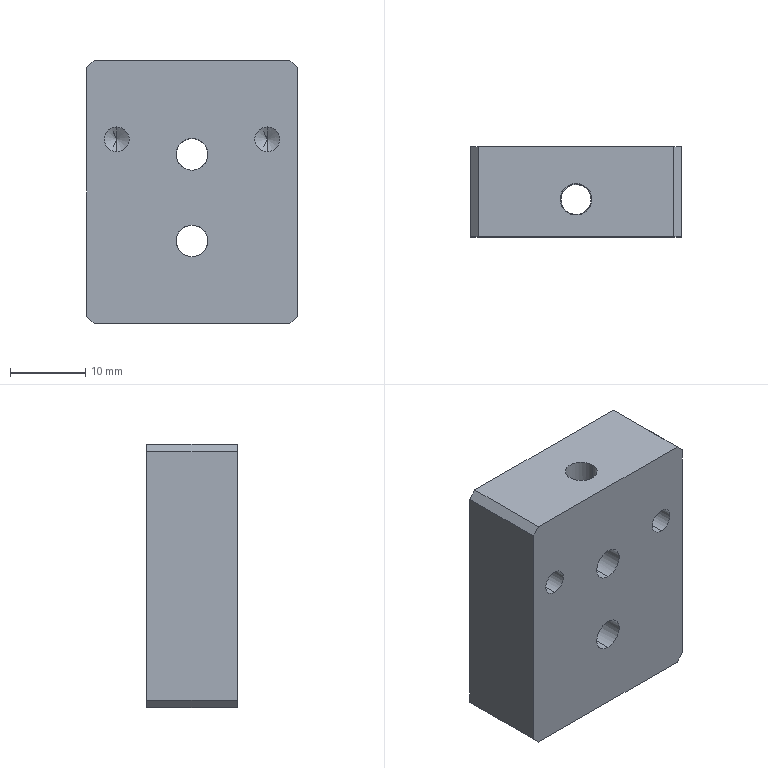Part | STEP file | 11-FG-E04411 | 1 solid | 36 faces | box 28 x 12 x 35 mm | volume 10850 mm3 | cylinder 19 | plane 10 | cone 7 | commonest cylinder face diameters 4.2 x13 3.3 x4 4 x2
STEP:
#1=CARTESIAN_POINT('',(-2.099,5.,5.1));
#2=VERTEX_POINT('',#1);
#3=CARTESIAN_POINT('',(-2.098,4.9,5.1));
#4=VERTEX_POINT('',#3);
#5=CARTESIAN_POINT('',(-2.099,5.,5.1));
#6=CARTESIAN_POINT('',(-2.098,4.967,5.1));
#7=CARTESIAN_POINT('',(-2.098,4.933,5.1));
#8=CARTESIAN_POINT('',(-2.098,4.9,5.1));
#9=B_SPLINE_CURVE_WITH_KNOTS('',3,(#5,#6,#7,#8),.UNSPECIFIED.,.F.,.F.,(4,4),(0.5,1.),.UNSPECIFIED.);
#10=EDGE_CURVE('',#2,#4,#9,.T.);
#11=ORIENTED_EDGE('',*,*,#10,.F.);
#12=CARTESIAN_POINT('',(-2.1,5.,17.5));
#13=VERTEX_POINT('',#12);
#14=CARTESIAN_POINT('',(-2.1,5.,17.5));
#15=DIRECTION('',(0.,0.,1.));
#16=VECTOR('',#15,1000.);
#17=LINE('',#14,#16);
#18=EDGE_CURVE('',#2,#13,#17,.T.);
#19=ORIENTED_EDGE('',*,*,#18,.T.);
#20=CARTESIAN_POINT('',(2.1,5.,17.5));
#21=VERTEX_POINT('',#20);
#22=CARTESIAN_POINT('',(0.,5.,17.5));
#23=DIRECTION('',(0.,0.,1.));
#24=DIRECTION('',(1.,0.,0.));
#25=AXIS2_PLACEMENT_3D('',#22,#23,#24);
#26=CIRCLE('',#25,2.1);
#27=EDGE_CURVE('',#13,#21,#26,.T.);
#28=ORIENTED_EDGE('',*,*,#27,.T.);
#29=CARTESIAN_POINT('',(2.099,5.,5.1));
#30=VERTEX_POINT('',#29);
#31=CARTESIAN_POINT('',(2.1,5.,17.5));
#32=DIRECTION('',(0.,0.,1.));
#33=VECTOR('',#32,1000.);
#34=LINE('',#31,#33);
#35=EDGE_CURVE('',#30,#21,#34,.T.);
#36=ORIENTED_EDGE('',*,*,#35,.F.);
#37=CARTESIAN_POINT('',(2.098,4.9,5.1));
#38=VERTEX_POINT('',#37);
#39=CARTESIAN_POINT('',(2.098,4.9,5.1));
#40=CARTESIAN_POINT('',(2.098,4.933,5.1));
#41=CARTESIAN_POINT('',(2.098,4.967,5.1));
#42=CARTESIAN_POINT('',(2.099,5.,5.1));
#43=B_SPLINE_CURVE_WITH_KNOTS('',3,(#39,#40,#41,#42),.UNSPECIFIED.,.F.,.F.,(4,4),(0.,0.5),.UNSPECIFIED.);
#44=EDGE_CURVE('',#38,#30,#43,.T.);
#45=ORIENTED_EDGE('',*,*,#44,.F.);
#46=CARTESIAN_POINT('',(0.,2.9,7.1));
#47=VERTEX_POINT('',#46);
#48=CARTESIAN_POINT('',(0.,2.9,7.1));
#49=CARTESIAN_POINT('',(1.184,2.9,7.1));
#50=CARTESIAN_POINT('',(2.041,3.717,6.283));
#51=CARTESIAN_POINT('',(2.098,4.9,5.1));
#52=(BOUNDED_CURVE()B_SPLINE_CURVE(3,(#48,#49,#50,#51),.UNSPECIFIED.,.F.,.F.)B_SPLINE_CURVE_WITH_KNOTS((4,4),(3.142,4.665),.UNSPECIFIED.)CURVE()GEOMETRIC_REPRESENTATION_ITEM()RATIONAL_B_SPLINE_CURVE((1.,0.8158,0.8158,1.))REPRESENTATION_ITEM(''));
#53=EDGE_CURVE('',#47,#38,#52,.T.);
#54=ORIENTED_EDGE('',*,*,#53,.F.);
#55=CARTESIAN_POINT('',(-2.098,4.9,5.1));
#56=CARTESIAN_POINT('',(-2.041,3.717,6.283));
#57=CARTESIAN_POINT('',(-1.184,2.9,7.1));
#58=CARTESIAN_POINT('',(0.,2.9,7.1));
#59=(BOUNDED_CURVE()B_SPLINE_CURVE(3,(#55,#56,#57,#58),.UNSPECIFIED.,.F.,.F.)B_SPLINE_CURVE_WITH_KNOTS((4,4),(1.618,3.142),.UNSPECIFIED.)CURVE()GEOMETRIC_REPRESENTATION_ITEM()RATIONAL_B_SPLINE_CURVE((1.,0.8158,0.8158,1.))REPRESENTATION_ITEM(''));
#60=EDGE_CURVE('',#4,#47,#59,.T.);
#61=ORIENTED_EDGE('',*,*,#60,.F.);
#62=EDGE_LOOP('',(#11,#19,#28,#36,#45,#54,#61));
#63=FACE_OUTER_BOUND('',#62,.T.);
#64=CARTESIAN_POINT('',(0.,5.,17.5));
#65=DIRECTION('',(0.,0.,1.));
#66=DIRECTION('',(1.,0.,0.));
#67=AXIS2_PLACEMENT_3D('',#64,#65,#66);
#68=CYLINDRICAL_SURFACE('',#67,2.1);
#69=ADVANCED_FACE('',(#63),#68,.F.);
#70=CARTESIAN_POINT('',(2.1,5.,-6.5));
#71=VERTEX_POINT('',#70);
#72=CARTESIAN_POINT('',(0.,2.9,-8.6));
#73=VERTEX_POINT('',#72);
#74=CARTESIAN_POINT('',(2.1,5.,-6.5));
#75=CARTESIAN_POINT('',(2.1,3.77,-7.73));
#76=CARTESIAN_POINT('',(1.23,2.9,-8.6));
#77=CARTESIAN_POINT('',(0.,2.9,-8.6));
#78=(BOUNDED_CURVE()B_SPLINE_CURVE(3,(#74,#75,#76,#77),.UNSPECIFIED.,.F.,.F.)B_SPLINE_CURVE_WITH_KNOTS((4,4),(1.571,3.142),.UNSPECIFIED.)CURVE()GEOMETRIC_REPRESENTATION_ITEM()RATIONAL_B_SPLINE_CURVE((1.,0.8047,0.8047,1.))REPRESENTATION_ITEM(''));
#79=EDGE_CURVE('',#71,#73,#78,.T.);
#80=ORIENTED_EDGE('',*,*,#79,.F.);
#81=CARTESIAN_POINT('',(2.1,5.,-17.5));
#82=VERTEX_POINT('',#81);
#83=CARTESIAN_POINT('',(2.1,5.,-17.5));
#84=DIRECTION('',(0.,0.,-1.));
#85=VECTOR('',#84,1000.);
#86=LINE('',#83,#85);
#87=EDGE_CURVE('',#71,#82,#86,.T.);
#88=ORIENTED_EDGE('',*,*,#87,.T.);
#89=CARTESIAN_POINT('',(-2.1,5.,-17.5));
#90=VERTEX_POINT('',#89);
#91=CARTESIAN_POINT('',(0.,5.,-17.5));
#92=DIRECTION('',(0.,0.,-1.));
#93=DIRECTION('',(-1.,0.,0.));
#94=AXIS2_PLACEMENT_3D('',#91,#92,#93);
#95=CIRCLE('',#94,2.1);
#96=EDGE_CURVE('',#82,#90,#95,.T.);
#97=ORIENTED_EDGE('',*,*,#96,.T.);
#98=CARTESIAN_POINT('',(-2.1,5.,-6.5));
#99=VERTEX_POINT('',#98);
#100=CARTESIAN_POINT('',(-2.1,5.,-17.5));
#101=DIRECTION('',(0.,0.,-1.));
#102=VECTOR('',#101,1000.);
#103=LINE('',#100,#102);
#104=EDGE_CURVE('',#99,#90,#103,.T.);
#105=ORIENTED_EDGE('',*,*,#104,.F.);
#106=CARTESIAN_POINT('',(0.,2.9,-8.6));
#107=CARTESIAN_POINT('',(-1.23,2.9,-8.6));
#108=CARTESIAN_POINT('',(-2.1,3.77,-7.73));
#109=CARTESIAN_POINT('',(-2.1,5.,-6.5));
#110=(BOUNDED_CURVE()B_SPLINE_CURVE(3,(#106,#107,#108,#109),.UNSPECIFIED.,.F.,.T.)B_SPLINE_CURVE_WITH_KNOTS((4,4),(3.142,4.712),.UNSPECIFIED.)CURVE()GEOMETRIC_REPRESENTATION_ITEM()RATIONAL_B_SPLINE_CURVE((1.,0.8047,0.8047,1.))REPRESENTATION_ITEM(''));
#111=EDGE_CURVE('',#73,#99,#110,.T.);
#112=ORIENTED_EDGE('',*,*,#111,.F.);
#113=EDGE_LOOP('',(#80,#88,#97,#105,#112));
#114=FACE_OUTER_BOUND('',#113,.T.);
#115=CARTESIAN_POINT('',(0.,5.,-17.5));
#116=DIRECTION('',(0.,0.,-1.));
#117=DIRECTION('',(-1.,0.,0.));
#118=AXIS2_PLACEMENT_3D('',#115,#116,#117);
#119=CYLINDRICAL_SURFACE('',#118,2.1);
#120=ADVANCED_FACE('',(#114),#119,.F.);
#121=CARTESIAN_POINT('',(-2.1,5.,-5.1));
#122=VERTEX_POINT('',#121);
#123=CARTESIAN_POINT('',(-1.565,6.4,-5.1));
#124=VERTEX_POINT('',#123);
#125=CARTESIAN_POINT('',(0.,5.,-5.1));
#126=DIRECTION('',(0.,0.,-1.));
#127=DIRECTION('',(-1.,0.,0.));
#128=AXIS2_PLACEMENT_3D('',#125,#126,#127);
#129=CIRCLE('',#128,2.1);
#130=EDGE_CURVE('',#122,#124,#129,.T.);
#131=ORIENTED_EDGE('',*,*,#130,.F.);
#132=CARTESIAN_POINT('',(-2.1,5.,-17.5));
#133=DIRECTION('',(0.,0.,-1.));
#134=VECTOR('',#133,1000.);
#135=LINE('',#132,#134);
#136=EDGE_CURVE('',#122,#99,#135,.T.);
#137=ORIENTED_EDGE('',*,*,#136,.T.);
#138=CARTESIAN_POINT('',(-1.565,6.4,-5.1));
#139=CARTESIAN_POINT('',(-1.914,6.011,-5.489));
#140=CARTESIAN_POINT('',(-2.1,5.522,-5.978));
#141=CARTESIAN_POINT('',(-2.1,5.,-6.5));
#142=(BOUNDED_CURVE()B_SPLINE_CURVE(3,(#138,#139,#140,#141),.UNSPECIFIED.,.F.,.F.)B_SPLINE_CURVE_WITH_KNOTS((4,4),(0.8411,1.571),.UNSPECIFIED.)CURVE()GEOMETRIC_REPRESENTATION_ITEM()RATIONAL_B_SPLINE_CURVE((1.,0.9561,0.9561,1.))REPRESENTATION_ITEM(''));
#143=EDGE_CURVE('',#124,#99,#142,.T.);
#144=ORIENTED_EDGE('',*,*,#143,.F.);
#145=EDGE_LOOP('',(#131,#137,#144));
#146=FACE_OUTER_BOUND('',#145,.T.);
#147=CARTESIAN_POINT('',(0.,5.,-17.5));
#148=DIRECTION('',(0.,0.,-1.));
#149=DIRECTION('',(-1.,0.,0.));
#150=AXIS2_PLACEMENT_3D('',#147,#148,#149);
#151=CYLINDRICAL_SURFACE('',#150,2.1);
#152=ADVANCED_FACE('',(#146),#151,.F.);
#153=CARTESIAN_POINT('',(-2.,5.,-5.04));
#154=VERTEX_POINT('',#153);
#155=CARTESIAN_POINT('',(-1.509,6.312,-5.04));
#156=VERTEX_POINT('',#155);
#157=CARTESIAN_POINT('',(0.,5.,-5.04));
#158=DIRECTION('',(0.,0.,-1.));
#159=DIRECTION('',(-1.,0.,0.));
#160=AXIS2_PLACEMENT_3D('',#157,#158,#159);
#161=CIRCLE('',#160,2.);
#162=EDGE_CURVE('',#154,#156,#161,.T.);
#163=ORIENTED_EDGE('',*,*,#162,.F.);
#164=CARTESIAN_POINT('',(-2.1,5.,-5.1));
#165=DIRECTION('',(-0.8572,0.,-0.515));
#166=VECTOR('',#165,1000.);
#167=LINE('',#164,#166);
#168=EDGE_CURVE('',#154,#122,#167,.T.);
#169=ORIENTED_EDGE('',*,*,#168,.T.);
#170=ORIENTED_EDGE('',*,*,#130,.T.);
#171=CARTESIAN_POINT('',(-1.509,6.312,-5.04));
#172=CARTESIAN_POINT('',(-1.529,6.341,-5.06));
#173=CARTESIAN_POINT('',(-1.547,6.37,-5.08));
#174=CARTESIAN_POINT('',(-1.565,6.4,-5.1));
#175=B_SPLINE_CURVE_WITH_KNOTS('',3,(#171,#172,#173,#174),.UNSPECIFIED.,.F.,.F.,(4,4),(0.003861,0.00398),.UNSPECIFIED.);
#176=EDGE_CURVE('',#156,#124,#175,.T.);
#177=ORIENTED_EDGE('',*,*,#176,.F.);
#178=EDGE_LOOP('',(#163,#169,#170,#177));
#179=FACE_OUTER_BOUND('',#178,.T.);
#180=CARTESIAN_POINT('',(0.,5.,-5.1));
#181=DIRECTION('',(0.,0.,-1.));
#182=DIRECTION('',(-1.,0.,0.));
#183=AXIS2_PLACEMENT_3D('',#180,#181,#182);
#184=CONICAL_SURFACE('',#183,2.1,1.03);
#185=ADVANCED_FACE('',(#179),#184,.F.);
#186=CARTESIAN_POINT('',(2.,5.,4.36));
#187=VERTEX_POINT('',#186);
#188=CARTESIAN_POINT('',(0.,3.,2.9));
#189=VERTEX_POINT('',#188);
#190=CARTESIAN_POINT('',(2.,5.,4.36));
#191=CARTESIAN_POINT('',(2.,4.926,4.36));
#192=CARTESIAN_POINT('',(1.996,4.852,4.346));
#193=CARTESIAN_POINT('',(1.98,4.712,4.301));
#194=CARTESIAN_POINT('',(1.969,4.645,4.27));
#195=CARTESIAN_POINT('',(1.929,4.455,4.166));
#196=CARTESIAN_POINT('',(1.892,4.34,4.083));
#197=CARTESIAN_POINT('',(1.799,4.118,3.913));
#198=CARTESIAN_POINT('',(1.744,4.013,3.825));
#199=CARTESIAN_POINT('',(1.615,3.815,3.654));
#200=CARTESIAN_POINT('',(1.542,3.721,3.57));
#201=CARTESIAN_POINT('',(1.375,3.543,3.409));
#202=CARTESIAN_POINT('',(1.281,3.458,3.331));
#203=CARTESIAN_POINT('',(1.073,3.307,3.19));
#204=CARTESIAN_POINT('',(0.959,3.24,3.127));
#205=CARTESIAN_POINT('',(0.7085,3.125,3.018));
#206=CARTESIAN_POINT('',(0.5753,3.079,2.975));
#207=CARTESIAN_POINT('',(0.294,3.016,2.916));
#208=CARTESIAN_POINT('',(0.1462,3.,2.9));
#209=CARTESIAN_POINT('',(0.,3.,2.9));
#210=B_SPLINE_CURVE_WITH_KNOTS('',3,(#190,#191,#192,#193,#194,#195,#196,#197,#198,#199,#200,#201,#202,#203,#204,#205,#206,#207,#208,#209),.UNSPECIFIED.,.F.,.F.,(4,2,2,2,2,2,2,2,2,4),(0.007048,0.00727,0.007491,0.007933,0.008376,0.008818,0.009261,0.009703,0.01015,0.01059),.UNSPECIFIED.);
#211=EDGE_CURVE('',#187,#189,#210,.T.);
#212=ORIENTED_EDGE('',*,*,#211,.F.);
#213=CARTESIAN_POINT('',(2.,5.,-5.04));
#214=VERTEX_POINT('',#213);
#215=CARTESIAN_POINT('',(2.,5.,21.5));
#216=DIRECTION('',(0.,0.,-1.));
#217=VECTOR('',#216,1000.);
#218=LINE('',#215,#217);
#219=EDGE_CURVE('',#187,#214,#218,.T.);
#220=ORIENTED_EDGE('',*,*,#219,.T.);
#221=CARTESIAN_POINT('',(1.509,3.688,-5.04));
#222=VERTEX_POINT('',#221);
#223=CARTESIAN_POINT('',(0.,5.,-5.04));
#224=DIRECTION('',(0.,0.,-1.));
#225=DIRECTION('',(-1.,0.,0.));
#226=AXIS2_PLACEMENT_3D('',#223,#224,#225);
#227=CIRCLE('',#226,2.);
#228=EDGE_CURVE('',#214,#222,#227,.T.);
#229=ORIENTED_EDGE('',*,*,#228,.T.);
#230=CARTESIAN_POINT('',(0.,3.,-4.4));
#231=VERTEX_POINT('',#230);
#232=CARTESIAN_POINT('',(0.,3.,-4.4));
#233=CARTESIAN_POINT('',(0.1564,3.,-4.4));
#234=CARTESIAN_POINT('',(0.3081,3.018,-4.417));
#235=CARTESIAN_POINT('',(0.603,3.087,-4.483));
#236=CARTESIAN_POINT('',(0.7432,3.138,-4.531));
#237=CARTESIAN_POINT('',(1.001,3.262,-4.648));
#238=CARTESIAN_POINT('',(1.119,3.337,-4.718));
#239=CARTESIAN_POINT('',(1.331,3.501,-4.87));
#240=CARTESIAN_POINT('',(1.425,3.591,-4.953));
#241=CARTESIAN_POINT('',(1.509,3.688,-5.04));
#242=B_SPLINE_CURVE_WITH_KNOTS('',3,(#232,#233,#234,#235,#236,#237,#238,#239,#240,#241),.UNSPECIFIED.,.F.,.F.,(4,2,2,2,4),(0.,0.0004611,0.0009223,0.001383,0.001845),.UNSPECIFIED.);
#243=EDGE_CURVE('',#231,#222,#242,.T.);
#244=ORIENTED_EDGE('',*,*,#243,.F.);
#245=CARTESIAN_POINT('',(-1.509,3.688,-5.04));
#246=VERTEX_POINT('',#245);
#247=CARTESIAN_POINT('',(-1.509,3.688,-5.04));
#248=CARTESIAN_POINT('',(-1.425,3.591,-4.953));
#249=CARTESIAN_POINT('',(-1.331,3.501,-4.87));
#250=CARTESIAN_POINT('',(-1.119,3.337,-4.718));
#251=CARTESIAN_POINT('',(-1.,3.262,-4.648));
#252=CARTESIAN_POINT('',(-0.7433,3.138,-4.531));
#253=CARTESIAN_POINT('',(-0.6036,3.087,-4.483));
#254=CARTESIAN_POINT('',(-0.3082,3.018,-4.417));
#255=CARTESIAN_POINT('',(-0.1571,3.,-4.4));
#256=CARTESIAN_POINT('',(0.,3.,-4.4));
#257=B_SPLINE_CURVE_WITH_KNOTS('',3,(#247,#248,#249,#250,#251,#252,#253,#254,#255,#256),.UNSPECIFIED.,.F.,.F.,(4,2,2,2,4),(0.01221,0.01268,0.01314,0.0136,0.01407),.UNSPECIFIED.);
#258=EDGE_CURVE('',#246,#231,#257,.T.);
#259=ORIENTED_EDGE('',*,*,#258,.F.);
#260=CARTESIAN_POINT('',(0.,5.,-5.04));
#261=DIRECTION('',(0.,0.,-1.));
#262=DIRECTION('',(-1.,0.,0.));
#263=AXIS2_PLACEMENT_3D('',#260,#261,#262);
#264=CIRCLE('',#263,2.);
#265=EDGE_CURVE('',#246,#154,#264,.T.);
#266=ORIENTED_EDGE('',*,*,#265,.T.);
#267=CARTESIAN_POINT('',(-2.,5.,4.36));
#268=VERTEX_POINT('',#267);
#269=CARTESIAN_POINT('',(-2.,5.,21.5));
#270=DIRECTION('',(0.,0.,-1.));
#271=VECTOR('',#270,1000.);
#272=LINE('',#269,#271);
#273=EDGE_CURVE('',#268,#154,#272,.T.);
#274=ORIENTED_EDGE('',*,*,#273,.F.);
#275=CARTESIAN_POINT('',(0.,3.,2.9));
#276=CARTESIAN_POINT('',(-0.146,3.,2.9));
#277=CARTESIAN_POINT('',(-0.2945,3.017,2.916));
#278=CARTESIAN_POINT('',(-0.5747,3.079,2.975));
#279=CARTESIAN_POINT('',(-0.7099,3.125,3.019));
#280=CARTESIAN_POINT('',(-0.9584,3.239,3.127));
#281=CARTESIAN_POINT('',(-1.073,3.308,3.191));
#282=CARTESIAN_POINT('',(-1.282,3.46,3.332));
#283=CARTESIAN_POINT('',(-1.375,3.542,3.408));
#284=CARTESIAN_POINT('',(-1.542,3.72,3.569));
#285=CARTESIAN_POINT('',(-1.616,3.816,3.655));
#286=CARTESIAN_POINT('',(-1.745,4.016,3.827));
#287=CARTESIAN_POINT('',(-1.8,4.12,3.914));
#288=CARTESIAN_POINT('',(-1.892,4.34,4.083));
#289=CARTESIAN_POINT('',(-1.929,4.457,4.167));
#290=CARTESIAN_POINT('',(-1.983,4.711,4.306));
#291=CARTESIAN_POINT('',(-2.,4.85,4.36));
#292=CARTESIAN_POINT('',(-2.,5.,4.36));
#293=B_SPLINE_CURVE_WITH_KNOTS('',3,(#275,#276,#277,#278,#279,#280,#281,#282,#283,#284,#285,#286,#287,#288,#289,#290,#291,#292),.UNSPECIFIED.,.F.,.F.,(4,2,2,2,2,2,2,2,4),(0.01059,0.01103,0.01147,0.01191,0.01236,0.0128,0.01324,0.01368,0.01412),.UNSPECIFIED.);
#294=EDGE_CURVE('',#189,#268,#293,.T.);
#295=ORIENTED_EDGE('',*,*,#294,.F.);
#296=EDGE_LOOP('',(#212,#220,#229,#244,#259,#266,#274,#295));
#297=FACE_OUTER_BOUND('',#296,.T.);
#298=CARTESIAN_POINT('',(0.,5.,21.5));
#299=DIRECTION('',(0.,0.,-1.));
#300=DIRECTION('',(-1.,0.,0.));
#301=AXIS2_PLACEMENT_3D('',#298,#299,#300);
#302=CYLINDRICAL_SURFACE('',#301,2.);
#303=ADVANCED_FACE('',(#297),#302,.F.);
#304=CARTESIAN_POINT('',(-10.,10.1,8.65));
#305=VERTEX_POINT('',#304);
#306=CARTESIAN_POINT('',(-10.,10.1,5.35));
#307=VERTEX_POINT('',#306);
#308=CARTESIAN_POINT('',(-10.,10.1,7.));
#309=DIRECTION('',(0.,-1.,0.));
#310=DIRECTION('',(0.,0.,-1.));
#311=AXIS2_PLACEMENT_3D('',#308,#309,#310);
#312=CIRCLE('',#311,1.65);
#313=EDGE_CURVE('',#305,#307,#312,.T.);
#314=ORIENTED_EDGE('',*,*,#313,.F.);
#315=CARTESIAN_POINT('',(-10.,0.,8.65));
#316=VERTEX_POINT('',#315);
#317=CARTESIAN_POINT('',(-10.,0.,8.65));
#318=DIRECTION('',(0.,-1.,0.));
#319=VECTOR('',#318,1000.);
#320=LINE('',#317,#319);
#321=EDGE_CURVE('',#305,#316,#320,.T.);
#322=ORIENTED_EDGE('',*,*,#321,.T.);
#323=CARTESIAN_POINT('',(-10.,0.,5.35));
#324=VERTEX_POINT('',#323);
#325=CARTESIAN_POINT('',(-10.,0.,7.));
#326=DIRECTION('',(0.,-1.,0.));
#327=DIRECTION('',(0.,0.,-1.));
#328=AXIS2_PLACEMENT_3D('',#325,#326,#327);
#329=CIRCLE('',#328,1.65);
#330=EDGE_CURVE('',#316,#324,#329,.T.);
#331=ORIENTED_EDGE('',*,*,#330,.T.);
#332=CARTESIAN_POINT('',(-10.,0.,5.35));
#333=DIRECTION('',(0.,-1.,0.));
#334=VECTOR('',#333,1000.);
#335=LINE('',#332,#334);
#336=EDGE_CURVE('',#307,#324,#335,.T.);
#337=ORIENTED_EDGE('',*,*,#336,.F.);
#338=EDGE_LOOP('',(#314,#322,#331,#337));
#339=FACE_OUTER_BOUND('',#338,.T.);
#340=CARTESIAN_POINT('',(-10.,0.,7.));
#341=DIRECTION('',(0.,-1.,0.));
#342=DIRECTION('',(0.,0.,-1.));
#343=AXIS2_PLACEMENT_3D('',#340,#341,#342);
#344=CYLINDRICAL_SURFACE('',#343,1.65);
#345=ADVANCED_FACE('',(#339),#344,.F.);
#346=CARTESIAN_POINT('',(-10.,11.091,7.));
#347=VERTEX_POINT('',#346);
#348=CARTESIAN_POINT('',(-10.,10.1,5.35));
#349=DIRECTION('',(0.,-0.515,-0.8572));
#350=VECTOR('',#349,1000.);
#351=LINE('',#348,#350);
#352=EDGE_CURVE('',#347,#307,#351,.T.);
#353=ORIENTED_EDGE('',*,*,#352,.F.);
#354=CARTESIAN_POINT('',(-10.,10.1,8.65));
#355=DIRECTION('',(0.,-0.515,0.8572));
#356=VECTOR('',#355,1000.);
#357=LINE('',#354,#356);
#358=EDGE_CURVE('',#347,#305,#357,.T.);
#359=ORIENTED_EDGE('',*,*,#358,.T.);
#360=ORIENTED_EDGE('',*,*,#313,.T.);
#361=EDGE_LOOP('',(#353,#359,#360));
#362=FACE_OUTER_BOUND('',#361,.T.);
#363=CARTESIAN_POINT('',(-10.,10.1,7.));
#364=DIRECTION('',(0.,-1.,0.));
#365=DIRECTION('',(0.,0.,-1.));
#366=AXIS2_PLACEMENT_3D('',#363,#364,#365);
#367=CONICAL_SURFACE('',#366,1.65,1.03);
#368=ADVANCED_FACE('',(#362),#367,.F.);
#369=CARTESIAN_POINT('',(10.,10.1,8.65));
#370=VERTEX_POINT('',#369);
#371=CARTESIAN_POINT('',(10.,10.1,5.35));
#372=VERTEX_POINT('',#371);
#373=CARTESIAN_POINT('',(10.,10.1,7.));
#374=DIRECTION('',(0.,-1.,0.));
#375=DIRECTION('',(0.,0.,-1.));
#376=AXIS2_PLACEMENT_3D('',#373,#374,#375);
#377=CIRCLE('',#376,1.65);
#378=EDGE_CURVE('',#370,#372,#377,.T.);
#379=ORIENTED_EDGE('',*,*,#378,.F.);
#380=CARTESIAN_POINT('',(10.,0.,8.65));
#381=VERTEX_POINT('',#380);
#382=CARTESIAN_POINT('',(10.,0.,8.65));
#383=DIRECTION('',(0.,-1.,0.));
#384=VECTOR('',#383,1000.);
#385=LINE('',#382,#384);
#386=EDGE_CURVE('',#370,#381,#385,.T.);
#387=ORIENTED_EDGE('',*,*,#386,.T.);
#388=CARTESIAN_POINT('',(10.,0.,5.35));
#389=VERTEX_POINT('',#388);
#390=CARTESIAN_POINT('',(10.,0.,7.));
#391=DIRECTION('',(0.,-1.,0.));
#392=DIRECTION('',(0.,0.,-1.));
#393=AXIS2_PLACEMENT_3D('',#390,#391,#392);
#394=CIRCLE('',#393,1.65);
#395=EDGE_CURVE('',#381,#389,#394,.T.);
#396=ORIENTED_EDGE('',*,*,#395,.T.);
#397=CARTESIAN_POINT('',(10.,0.,5.35));
#398=DIRECTION('',(0.,-1.,0.));
#399=VECTOR('',#398,1000.);
#400=LINE('',#397,#399);
#401=EDGE_CURVE('',#372,#389,#400,.T.);
#402=ORIENTED_EDGE('',*,*,#401,.F.);
#403=EDGE_LOOP('',(#379,#387,#396,#402));
#404=FACE_OUTER_BOUND('',#403,.T.);
#405=CARTESIAN_POINT('',(10.,0.,7.));
#406=DIRECTION('',(0.,-1.,0.));
#407=DIRECTION('',(0.,0.,-1.));
#408=AXIS2_PLACEMENT_3D('',#405,#406,#407);
#409=CYLINDRICAL_SURFACE('',#408,1.65);
#410=ADVANCED_FACE('',(#404),#409,.F.);
#411=CARTESIAN_POINT('',(10.,11.091,7.));
#412=VERTEX_POINT('',#411);
#413=CARTESIAN_POINT('',(10.,10.1,5.35));
#414=DIRECTION('',(0.,-0.515,-0.8572));
#415=VECTOR('',#414,1000.);
#416=LINE('',#413,#415);
#417=EDGE_CURVE('',#412,#372,#416,.T.);
#418=ORIENTED_EDGE('',*,*,#417,.F.);
#419=CARTESIAN_POINT('',(10.,10.1,8.65));
#420=DIRECTION('',(0.,-0.515,0.8572));
#421=VECTOR('',#420,1000.);
#422=LINE('',#419,#421);
#423=EDGE_CURVE('',#412,#370,#422,.T.);
#424=ORIENTED_EDGE('',*,*,#423,.T.);
#425=ORIENTED_EDGE('',*,*,#378,.T.);
#426=EDGE_LOOP('',(#418,#424,#425));
#427=FACE_OUTER_BOUND('',#426,.T.);
#428=CARTESIAN_POINT('',(10.,10.1,7.));
#429=DIRECTION('',(0.,-1.,0.));
#430=DIRECTION('',(0.,0.,-1.));
#431=AXIS2_PLACEMENT_3D('',#428,#429,#430);
#432=CONICAL_SURFACE('',#431,1.65,1.03);
#433=ADVANCED_FACE('',(#427),#432,.F.);
#434=CARTESIAN_POINT('',(0.,7.1,-8.6));
#435=VERTEX_POINT('',#434);
#436=CARTESIAN_POINT('',(-2.1,5.,-6.5));
#437=CARTESIAN_POINT('',(-2.1,6.23,-7.73));
#438=CARTESIAN_POINT('',(-1.23,7.1,-8.6));
#439=CARTESIAN_POINT('',(0.,7.1,-8.6));
#440=(BOUNDED_CURVE()B_SPLINE_CURVE(3,(#436,#437,#438,#439),.UNSPECIFIED.,.F.,.F.)B_SPLINE_CURVE_WITH_KNOTS((4,4),(4.712,6.283),.UNSPECIFIED.)CURVE()GEOMETRIC_REPRESENTATION_ITEM()RATIONAL_B_SPLINE_CURVE((1.,0.8047,0.8047,1.))REPRESENTATION_ITEM(''));
#441=EDGE_CURVE('',#99,#435,#440,.T.);
#442=ORIENTED_EDGE('',*,*,#441,.T.);
#443=CARTESIAN_POINT('',(0.,12.,-8.6));
#444=VERTEX_POINT('',#443);
#445=CARTESIAN_POINT('',(0.,12.,-8.6));
#446=DIRECTION('',(0.,1.,0.));
#447=VECTOR('',#446,1000.);
#448=LINE('',#445,#447);
#449=EDGE_CURVE('',#435,#444,#448,.T.);
#450=ORIENTED_EDGE('',*,*,#449,.T.);
#451=CARTESIAN_POINT('',(0.,12.,-4.4));
#452=VERTEX_POINT('',#451);
#453=CARTESIAN_POINT('',(0.,12.,-6.5));
#454=DIRECTION('',(0.,1.,0.));
#455=DIRECTION('',(0.,0.,1.));
#456=AXIS2_PLACEMENT_3D('',#453,#454,#455);
#457=CIRCLE('',#456,2.1);
#458=EDGE_CURVE('',#444,#452,#457,.T.);
#459=ORIENTED_EDGE('',*,*,#458,.T.);
#460=CARTESIAN_POINT('',(0.,7.,-4.4));
#461=VERTEX_POINT('',#460);
#462=CARTESIAN_POINT('',(0.,12.,-4.4));
#463=DIRECTION('',(0.,1.,0.));
#464=VECTOR('',#463,1000.);
#465=LINE('',#462,#464);
#466=EDGE_CURVE('',#461,#452,#465,.T.);
#467=ORIENTED_EDGE('',*,*,#466,.F.);
#468=CARTESIAN_POINT('',(0.,7.,-4.4));
#469=CARTESIAN_POINT('',(-0.1553,7.,-4.4));
#470=CARTESIAN_POINT('',(-0.3073,6.982,-4.417));
#471=CARTESIAN_POINT('',(-0.6044,6.913,-4.483));
#472=CARTESIAN_POINT('',(-0.7426,6.863,-4.531));
#473=CARTESIAN_POINT('',(-1.002,6.737,-4.649));
#474=CARTESIAN_POINT('',(-1.119,6.663,-4.718));
#475=CARTESIAN_POINT('',(-1.33,6.5,-4.87));
#476=CARTESIAN_POINT('',(-1.426,6.408,-4.953));
#477=CARTESIAN_POINT('',(-1.509,6.312,-5.04));
#478=B_SPLINE_CURVE_WITH_KNOTS('',3,(#468,#469,#470,#471,#472,#473,#474,#475,#476,#477),.UNSPECIFIED.,.F.,.F.,(4,2,2,2,4),(0.007029,0.007491,0.007954,0.008416,0.008878),.UNSPECIFIED.);
#479=EDGE_CURVE('',#461,#156,#478,.T.);
#480=ORIENTED_EDGE('',*,*,#479,.T.);
#481=ORIENTED_EDGE('',*,*,#176,.T.);
#482=ORIENTED_EDGE('',*,*,#143,.T.);
#483=EDGE_LOOP('',(#442,#450,#459,#467,#480,#481,#482));
#484=FACE_OUTER_BOUND('',#483,.T.);
#485=CARTESIAN_POINT('',(0.,12.,-6.5));
#486=DIRECTION('',(0.,1.,0.));
#487=DIRECTION('',(0.,0.,1.));
#488=AXIS2_PLACEMENT_3D('',#485,#486,#487);
#489=CYLINDRICAL_SURFACE('',#488,2.1);
#490=ADVANCED_FACE('',(#484),#489,.F.);
#491=CARTESIAN_POINT('',(0.,0.,2.9));
#492=VERTEX_POINT('',#491);
#493=CARTESIAN_POINT('',(0.,0.,7.1));
#494=VERTEX_POINT('',#493);
#495=CARTESIAN_POINT('',(0.,0.,5.));
#496=DIRECTION('',(0.,1.,0.));
#497=DIRECTION('',(0.,0.,1.));
#498=AXIS2_PLACEMENT_3D('',#495,#496,#497);
#499=CIRCLE('',#498,2.1);
#500=EDGE_CURVE('',#492,#494,#499,.T.);
#501=ORIENTED_EDGE('',*,*,#500,.F.);
#502=CARTESIAN_POINT('',(0.,12.,2.9));
#503=DIRECTION('',(0.,1.,0.));
#504=VECTOR('',#503,1000.);
#505=LINE('',#502,#504);
#506=EDGE_CURVE('',#492,#189,#505,.T.);
#507=ORIENTED_EDGE('',*,*,#506,.T.);
#508=ORIENTED_EDGE('',*,*,#294,.T.);
#509=CARTESIAN_POINT('',(0.,7.,2.9));
#510=VERTEX_POINT('',#509);
#511=CARTESIAN_POINT('',(-2.,5.,4.36));
#512=CARTESIAN_POINT('',(-2.,5.15,4.36));
#513=CARTESIAN_POINT('',(-1.983,5.29,4.305));
#514=CARTESIAN_POINT('',(-1.929,5.544,4.167));
#515=CARTESIAN_POINT('',(-1.891,5.661,4.082));
#516=CARTESIAN_POINT('',(-1.799,5.881,3.913));
#517=CARTESIAN_POINT('',(-1.744,5.985,3.826));
#518=CARTESIAN_POINT('',(-1.616,6.185,3.654));
#519=CARTESIAN_POINT('',(-1.541,6.281,3.569));
#520=CARTESIAN_POINT('',(-1.374,6.459,3.407));
#521=CARTESIAN_POINT('',(-1.281,6.542,3.331));
#522=CARTESIAN_POINT('',(-1.072,6.693,3.19));
#523=CARTESIAN_POINT('',(-0.9564,6.762,3.126));
#524=CARTESIAN_POINT('',(-0.7086,6.875,3.019));
#525=CARTESIAN_POINT('',(-0.5729,6.922,2.975));
#526=CARTESIAN_POINT('',(-0.2927,6.984,2.916));
#527=CARTESIAN_POINT('',(-0.1486,7.,2.9));
#528=CARTESIAN_POINT('',(0.,7.,2.9));
#529=B_SPLINE_CURVE_WITH_KNOTS('',3,(#511,#512,#513,#514,#515,#516,#517,#518,#519,#520,#521,#522,#523,#524,#525,#526,#527,#528),.UNSPECIFIED.,.F.,.F.,(4,2,2,2,2,2,2,2,4),(0.,0.0004408,0.0008816,0.001322,0.001763,0.002204,0.002645,0.003085,0.003526),.UNSPECIFIED.);
#530=EDGE_CURVE('',#268,#510,#529,.T.);
#531=ORIENTED_EDGE('',*,*,#530,.T.);
#532=CARTESIAN_POINT('',(0.,12.,2.9));
#533=VERTEX_POINT('',#532);
#534=CARTESIAN_POINT('',(0.,12.,2.9));
#535=DIRECTION('',(0.,1.,0.));
#536=VECTOR('',#535,1000.);
#537=LINE('',#534,#536);
#538=EDGE_CURVE('',#510,#533,#537,.T.);
#539=ORIENTED_EDGE('',*,*,#538,.T.);
#540=CARTESIAN_POINT('',(0.,12.,7.1));
#541=VERTEX_POINT('',#540);
#542=CARTESIAN_POINT('',(0.,12.,5.));
#543=DIRECTION('',(0.,1.,0.));
#544=DIRECTION('',(0.,0.,1.));
#545=AXIS2_PLACEMENT_3D('',#542,#543,#544);
#546=CIRCLE('',#545,2.1);
#547=EDGE_CURVE('',#533,#541,#546,.T.);
#548=ORIENTED_EDGE('',*,*,#547,.T.);
#549=CARTESIAN_POINT('',(0.,7.1,7.1));
#550=VERTEX_POINT('',#549);
#551=CARTESIAN_POINT('',(0.,12.,7.1));
#552=DIRECTION('',(0.,1.,0.));
#553=VECTOR('',#552,1000.);
#554=LINE('',#551,#553);
#555=EDGE_CURVE('',#550,#541,#554,.T.);
#556=ORIENTED_EDGE('',*,*,#555,.F.);
#557=CARTESIAN_POINT('',(-2.098,5.1,5.1));
#558=VERTEX_POINT('',#557);
#559=CARTESIAN_POINT('',(0.,7.1,7.1));
#560=CARTESIAN_POINT('',(-1.184,7.1,7.1));
#561=CARTESIAN_POINT('',(-2.041,6.283,6.283));
#562=CARTESIAN_POINT('',(-2.098,5.1,5.1));
#563=(BOUNDED_CURVE()B_SPLINE_CURVE(3,(#559,#560,#561,#562),.UNSPECIFIED.,.F.,.F.)B_SPLINE_CURVE_WITH_KNOTS((4,4),(0.,1.523),.UNSPECIFIED.)CURVE()GEOMETRIC_REPRESENTATION_ITEM()RATIONAL_B_SPLINE_CURVE((1.,0.8158,0.8158,1.))REPRESENTATION_ITEM(''));
#564=EDGE_CURVE('',#550,#558,#563,.T.);
#565=ORIENTED_EDGE('',*,*,#564,.T.);
#566=CARTESIAN_POINT('',(-2.098,5.1,5.1));
#567=CARTESIAN_POINT('',(-2.098,5.067,5.1));
#568=CARTESIAN_POINT('',(-2.098,5.033,5.1));
#569=CARTESIAN_POINT('',(-2.099,5.,5.1));
#570=B_SPLINE_CURVE_WITH_KNOTS('',3,(#566,#567,#568,#569),.UNSPECIFIED.,.F.,.F.,(4,4),(0.,0.5),.UNSPECIFIED.);
#571=EDGE_CURVE('',#558,#2,#570,.T.);
#572=ORIENTED_EDGE('',*,*,#571,.T.);
#573=ORIENTED_EDGE('',*,*,#10,.T.);
#574=ORIENTED_EDGE('',*,*,#60,.T.);
#575=CARTESIAN_POINT('',(0.,12.,7.1));
#576=DIRECTION('',(0.,1.,0.));
#577=VECTOR('',#576,1000.);
#578=LINE('',#575,#577);
#579=EDGE_CURVE('',#494,#47,#578,.T.);
#580=ORIENTED_EDGE('',*,*,#579,.F.);
#581=EDGE_LOOP('',(#501,#507,#508,#531,#539,#548,#556,#565,#572,#573,#574,#580));
#582=FACE_OUTER_BOUND('',#581,.T.);
#583=CARTESIAN_POINT('',(0.,12.,5.));
#584=DIRECTION('',(0.,1.,0.));
#585=DIRECTION('',(0.,0.,1.));
#586=AXIS2_PLACEMENT_3D('',#583,#584,#585);
#587=CYLINDRICAL_SURFACE('',#586,2.1);
#588=ADVANCED_FACE('',(#582),#587,.F.);
#589=CARTESIAN_POINT('',(0.,0.,-8.6));
#590=VERTEX_POINT('',#589);
#591=CARTESIAN_POINT('',(0.,0.,-4.4));
#592=VERTEX_POINT('',#591);
#593=CARTESIAN_POINT('',(0.,0.,-6.5));
#594=DIRECTION('',(0.,1.,0.));
#595=DIRECTION('',(0.,0.,1.));
#596=AXIS2_PLACEMENT_3D('',#593,#594,#595);
#597=CIRCLE('',#596,2.1);
#598=EDGE_CURVE('',#590,#592,#597,.T.);
#599=ORIENTED_EDGE('',*,*,#598,.F.);
#600=CARTESIAN_POINT('',(0.,12.,-8.6));
#601=DIRECTION('',(0.,1.,0.));
#602=VECTOR('',#601,1000.);
#603=LINE('',#600,#602);
#604=EDGE_CURVE('',#590,#73,#603,.T.);
#605=ORIENTED_EDGE('',*,*,#604,.T.);
#606=ORIENTED_EDGE('',*,*,#111,.T.);
#607=CARTESIAN_POINT('',(-1.565,3.6,-5.1));
#608=VERTEX_POINT('',#607);
#609=CARTESIAN_POINT('',(-2.1,5.,-6.5));
#610=CARTESIAN_POINT('',(-2.1,4.478,-5.978));
#611=CARTESIAN_POINT('',(-1.914,3.989,-5.489));
#612=CARTESIAN_POINT('',(-1.565,3.6,-5.1));
#613=(BOUNDED_CURVE()B_SPLINE_CURVE(3,(#609,#610,#611,#612),.UNSPECIFIED.,.F.,.F.)B_SPLINE_CURVE_WITH_KNOTS((4,4),(1.571,2.301),.UNSPECIFIED.)CURVE()GEOMETRIC_REPRESENTATION_ITEM()RATIONAL_B_SPLINE_CURVE((1.,0.9561,0.9561,1.))REPRESENTATION_ITEM(''));
#614=EDGE_CURVE('',#99,#608,#613,.T.);
#615=ORIENTED_EDGE('',*,*,#614,.T.);
#616=CARTESIAN_POINT('',(-1.565,3.6,-5.1));
#617=CARTESIAN_POINT('',(-1.547,3.63,-5.08));
#618=CARTESIAN_POINT('',(-1.529,3.659,-5.06));
#619=CARTESIAN_POINT('',(-1.509,3.688,-5.04));
#620=B_SPLINE_CURVE_WITH_KNOTS('',3,(#616,#617,#618,#619),.UNSPECIFIED.,.F.,.F.,(4,4),(0.000141,0.000261),.UNSPECIFIED.);
#621=EDGE_CURVE('',#608,#246,#620,.T.);
#622=ORIENTED_EDGE('',*,*,#621,.T.);
#623=ORIENTED_EDGE('',*,*,#258,.T.);
#624=CARTESIAN_POINT('',(0.,12.,-4.4));
#625=DIRECTION('',(0.,1.,0.));
#626=VECTOR('',#625,1000.);
#627=LINE('',#624,#626);
#628=EDGE_CURVE('',#592,#231,#627,.T.);
#629=ORIENTED_EDGE('',*,*,#628,.F.);
#630=EDGE_LOOP('',(#599,#605,#606,#615,#622,#623,#629));
#631=FACE_OUTER_BOUND('',#630,.T.);
#632=CARTESIAN_POINT('',(0.,12.,-6.5));
#633=DIRECTION('',(0.,1.,0.));
#634=DIRECTION('',(0.,0.,1.));
#635=AXIS2_PLACEMENT_3D('',#632,#633,#634);
#636=CYLINDRICAL_SURFACE('',#635,2.1);
#637=ADVANCED_FACE('',(#631),#636,.F.);
#638=ORIENTED_EDGE('',*,*,#604,.F.);
#639=CARTESIAN_POINT('',(0.,0.,-6.5));
#640=DIRECTION('',(0.,1.,0.));
#641=DIRECTION('',(0.,0.,1.));
#642=AXIS2_PLACEMENT_3D('',#639,#640,#641);
#643=CIRCLE('',#642,2.1);
#644=EDGE_CURVE('',#592,#590,#643,.T.);
#645=ORIENTED_EDGE('',*,*,#644,.F.);
#646=ORIENTED_EDGE('',*,*,#628,.T.);
#647=ORIENTED_EDGE('',*,*,#243,.T.);
#648=CARTESIAN_POINT('',(1.565,3.6,-5.1));
#649=VERTEX_POINT('',#648);
#650=CARTESIAN_POINT('',(1.509,3.688,-5.04));
#651=CARTESIAN_POINT('',(1.529,3.659,-5.06));
#652=CARTESIAN_POINT('',(1.547,3.63,-5.08));
#653=CARTESIAN_POINT('',(1.565,3.6,-5.1));
#654=B_SPLINE_CURVE_WITH_KNOTS('',3,(#650,#651,#652,#653),.UNSPECIFIED.,.F.,.F.,(4,4),(0.003861,0.00398),.UNSPECIFIED.);
#655=EDGE_CURVE('',#222,#649,#654,.T.);
#656=ORIENTED_EDGE('',*,*,#655,.T.);
#657=CARTESIAN_POINT('',(1.565,3.6,-5.1));
#658=CARTESIAN_POINT('',(1.914,3.989,-5.489));
#659=CARTESIAN_POINT('',(2.1,4.478,-5.978));
#660=CARTESIAN_POINT('',(2.1,5.,-6.5));
#661=(BOUNDED_CURVE()B_SPLINE_CURVE(3,(#657,#658,#659,#660),.UNSPECIFIED.,.F.,.F.)B_SPLINE_CURVE_WITH_KNOTS((4,4),(3.983,4.712),.UNSPECIFIED.)CURVE()GEOMETRIC_REPRESENTATION_ITEM()RATIONAL_B_SPLINE_CURVE((1.,0.9561,0.9561,1.))REPRESENTATION_ITEM(''));
#662=EDGE_CURVE('',#649,#71,#661,.T.);
#663=ORIENTED_EDGE('',*,*,#662,.T.);
#664=ORIENTED_EDGE('',*,*,#79,.T.);
#665=EDGE_LOOP('',(#638,#645,#646,#647,#656,#663,#664));
#666=FACE_OUTER_BOUND('',#665,.T.);
#667=CARTESIAN_POINT('',(0.,12.,-6.5));
#668=DIRECTION('',(0.,1.,0.));
#669=DIRECTION('',(0.,0.,1.));
#670=AXIS2_PLACEMENT_3D('',#667,#668,#669);
#671=CYLINDRICAL_SURFACE('',#670,2.1);
#672=ADVANCED_FACE('',(#666),#671,.F.);
#673=CARTESIAN_POINT('',(14.,12.,16.5));
#674=VERTEX_POINT('',#673);
#675=CARTESIAN_POINT('',(14.,12.,-16.5));
#676=VERTEX_POINT('',#675);
#677=CARTESIAN_POINT('',(14.,12.,-17.5));
#678=DIRECTION('',(0.,0.,-1.));
#679=VECTOR('',#678,1000.);
#680=LINE('',#677,#679);
#681=EDGE_CURVE('',#674,#676,#680,.T.);
#682=ORIENTED_EDGE('',*,*,#681,.F.);
#683=CARTESIAN_POINT('',(14.,0.,16.5));
#684=VERTEX_POINT('',#683);
#685=CARTESIAN_POINT('',(14.,12.,16.5));
#686=DIRECTION('',(0.,-1.,0.));
#687=VECTOR('',#686,1000.);
#688=LINE('',#685,#687);
#689=EDGE_CURVE('',#674,#684,#688,.T.);
#690=ORIENTED_EDGE('',*,*,#689,.T.);
#691=CARTESIAN_POINT('',(14.,0.,-16.5));
#692=VERTEX_POINT('',#691);
#693=CARTESIAN_POINT('',(14.,0.,-17.5));
#694=DIRECTION('',(0.,0.,-1.));
#695=VECTOR('',#694,1000.);
#696=LINE('',#693,#695);
#697=EDGE_CURVE('',#684,#692,#696,.T.);
#698=ORIENTED_EDGE('',*,*,#697,.T.);
#699=CARTESIAN_POINT('',(14.,12.,-16.5));
#700=DIRECTION('',(0.,1.,0.));
#701=VECTOR('',#700,1000.);
#702=LINE('',#699,#701);
#703=EDGE_CURVE('',#692,#676,#702,.T.);
#704=ORIENTED_EDGE('',*,*,#703,.T.);
#705=EDGE_LOOP('',(#682,#690,#698,#704));
#706=FACE_OUTER_BOUND('',#705,.T.);
#707=CARTESIAN_POINT('',(14.,12.,-17.5));
#708=DIRECTION('',(-1.,0.,0.));
#709=DIRECTION('',(0.,0.,1.));
#710=AXIS2_PLACEMENT_3D('',#707,#708,#709);
#711=PLANE('',#710);
#712=ADVANCED_FACE('',(#706),#711,.F.);
#713=CARTESIAN_POINT('',(0.,5.,-17.5));
#714=DIRECTION('',(0.,0.,-1.));
#715=DIRECTION('',(-1.,0.,0.));
#716=AXIS2_PLACEMENT_3D('',#713,#714,#715);
#717=CIRCLE('',#716,2.1);
#718=EDGE_CURVE('',#90,#82,#717,.T.);
#719=ORIENTED_EDGE('',*,*,#718,.F.);
#720=ORIENTED_EDGE('',*,*,#96,.F.);
#721=EDGE_LOOP('',(#719,#720));
#722=FACE_BOUND('',#721,.T.);
#723=CARTESIAN_POINT('',(13.,0.,-17.5));
#724=VERTEX_POINT('',#723);
#725=CARTESIAN_POINT('',(-13.,0.,-17.5));
#726=VERTEX_POINT('',#725);
#727=CARTESIAN_POINT('',(-14.,0.,-17.5));
#728=DIRECTION('',(-1.,0.,0.));
#729=VECTOR('',#728,1000.);
#730=LINE('',#727,#729);
#731=EDGE_CURVE('',#724,#726,#730,.T.);
#732=ORIENTED_EDGE('',*,*,#731,.T.);
#733=CARTESIAN_POINT('',(-13.,12.,-17.5));
#734=VERTEX_POINT('',#733);
#735=CARTESIAN_POINT('',(-13.,12.,-17.5));
#736=DIRECTION('',(0.,1.,0.));
#737=VECTOR('',#736,1000.);
#738=LINE('',#735,#737);
#739=EDGE_CURVE('',#726,#734,#738,.T.);
#740=ORIENTED_EDGE('',*,*,#739,.T.);
#741=CARTESIAN_POINT('',(13.,12.,-17.5));
#742=VERTEX_POINT('',#741);
#743=CARTESIAN_POINT('',(-14.,12.,-17.5));
#744=DIRECTION('',(-1.,0.,0.));
#745=VECTOR('',#744,1000.);
#746=LINE('',#743,#745);
#747=EDGE_CURVE('',#742,#734,#746,.T.);
#748=ORIENTED_EDGE('',*,*,#747,.F.);
#749=CARTESIAN_POINT('',(13.,12.,-17.5));
#750=DIRECTION('',(0.,-1.,0.));
#751=VECTOR('',#750,1000.);
#752=LINE('',#749,#751);
#753=EDGE_CURVE('',#742,#724,#752,.T.);
#754=ORIENTED_EDGE('',*,*,#753,.T.);
#755=EDGE_LOOP('',(#732,#740,#748,#754));
#756=FACE_OUTER_BOUND('',#755,.T.);
#757=CARTESIAN_POINT('',(-14.,12.,-17.5));
#758=DIRECTION('',(0.,0.,1.));
#759=DIRECTION('',(1.,0.,0.));
#760=AXIS2_PLACEMENT_3D('',#757,#758,#759);
#761=PLANE('',#760);
#762=ADVANCED_FACE('',(#722,#756),#761,.F.);
#763=CARTESIAN_POINT('',(-14.,0.,-16.5));
#764=VERTEX_POINT('',#763);
#765=CARTESIAN_POINT('',(-14.,0.,16.5));
#766=VERTEX_POINT('',#765);
#767=CARTESIAN_POINT('',(-14.,0.,-17.5));
#768=DIRECTION('',(0.,0.,1.));
#769=VECTOR('',#768,1000.);
#770=LINE('',#767,#769);
#771=EDGE_CURVE('',#764,#766,#770,.T.);
#772=ORIENTED_EDGE('',*,*,#771,.T.);
#773=CARTESIAN_POINT('',(-14.,12.,16.5));
#774=VERTEX_POINT('',#773);
#775=CARTESIAN_POINT('',(-14.,12.,16.5));
#776=DIRECTION('',(0.,1.,0.));
#777=VECTOR('',#776,1000.);
#778=LINE('',#775,#777);
#779=EDGE_CURVE('',#766,#774,#778,.T.);
#780=ORIENTED_EDGE('',*,*,#779,.T.);
#781=CARTESIAN_POINT('',(-14.,12.,-16.5));
#782=VERTEX_POINT('',#781);
#783=CARTESIAN_POINT('',(-14.,12.,-17.5));
#784=DIRECTION('',(0.,0.,1.));
#785=VECTOR('',#784,1000.);
#786=LINE('',#783,#785);
#787=EDGE_CURVE('',#782,#774,#786,.T.);
#788=ORIENTED_EDGE('',*,*,#787,.F.);
#789=CARTESIAN_POINT('',(-14.,12.,-16.5));
#790=DIRECTION('',(0.,-1.,0.));
#791=VECTOR('',#790,1000.);
#792=LINE('',#789,#791);
#793=EDGE_CURVE('',#782,#764,#792,.T.);
#794=ORIENTED_EDGE('',*,*,#793,.T.);
#795=EDGE_LOOP('',(#772,#780,#788,#794));
#796=FACE_OUTER_BOUND('',#795,.T.);
#797=CARTESIAN_POINT('',(-14.,12.,-17.5));
#798=DIRECTION('',(1.,0.,0.));
#799=DIRECTION('',(0.,0.,-1.));
#800=AXIS2_PLACEMENT_3D('',#797,#798,#799);
#801=PLANE('',#800);
#802=ADVANCED_FACE('',(#796),#801,.F.);
#803=CARTESIAN_POINT('',(0.,5.,17.5));
#804=DIRECTION('',(0.,0.,1.));
#805=DIRECTION('',(1.,0.,0.));
#806=AXIS2_PLACEMENT_3D('',#803,#804,#805);
#807=CIRCLE('',#806,2.1);
#808=EDGE_CURVE('',#21,#13,#807,.T.);
#809=ORIENTED_EDGE('',*,*,#808,.F.);
#810=ORIENTED_EDGE('',*,*,#27,.F.);
#811=EDGE_LOOP('',(#809,#810));
#812=FACE_BOUND('',#811,.T.);
#813=CARTESIAN_POINT('',(-13.,0.,17.5));
#814=VERTEX_POINT('',#813);
#815=CARTESIAN_POINT('',(13.,0.,17.5));
#816=VERTEX_POINT('',#815);
#817=CARTESIAN_POINT('',(-14.,0.,17.5));
#818=DIRECTION('',(1.,0.,0.));
#819=VECTOR('',#818,1000.);
#820=LINE('',#817,#819);
#821=EDGE_CURVE('',#814,#816,#820,.T.);
#822=ORIENTED_EDGE('',*,*,#821,.T.);
#823=CARTESIAN_POINT('',(13.,12.,17.5));
#824=VERTEX_POINT('',#823);
#825=CARTESIAN_POINT('',(13.,12.,17.5));
#826=DIRECTION('',(0.,1.,0.));
#827=VECTOR('',#826,1000.);
#828=LINE('',#825,#827);
#829=EDGE_CURVE('',#816,#824,#828,.T.);
#830=ORIENTED_EDGE('',*,*,#829,.T.);
#831=CARTESIAN_POINT('',(-13.,12.,17.5));
#832=VERTEX_POINT('',#831);
#833=CARTESIAN_POINT('',(-14.,12.,17.5));
#834=DIRECTION('',(1.,0.,0.));
#835=VECTOR('',#834,1000.);
#836=LINE('',#833,#835);
#837=EDGE_CURVE('',#832,#824,#836,.T.);
#838=ORIENTED_EDGE('',*,*,#837,.F.);
#839=CARTESIAN_POINT('',(-13.,12.,17.5));
#840=DIRECTION('',(0.,-1.,0.));
#841=VECTOR('',#840,1000.);
#842=LINE('',#839,#841);
#843=EDGE_CURVE('',#832,#814,#842,.T.);
#844=ORIENTED_EDGE('',*,*,#843,.T.);
#845=EDGE_LOOP('',(#822,#830,#838,#844));
#846=FACE_OUTER_BOUND('',#845,.T.);
#847=CARTESIAN_POINT('',(-14.,12.,17.5));
#848=DIRECTION('',(0.,0.,-1.));
#849=DIRECTION('',(-1.,0.,0.));
#850=AXIS2_PLACEMENT_3D('',#847,#848,#849);
#851=PLANE('',#850);
#852=ADVANCED_FACE('',(#812,#846),#851,.F.);
#853=CARTESIAN_POINT('',(0.,12.,-6.5));
#854=DIRECTION('',(0.,1.,0.));
#855=DIRECTION('',(0.,0.,1.));
#856=AXIS2_PLACEMENT_3D('',#853,#854,#855);
#857=CIRCLE('',#856,2.1);
#858=EDGE_CURVE('',#452,#444,#857,.T.);
#859=ORIENTED_EDGE('',*,*,#858,.F.);
#860=ORIENTED_EDGE('',*,*,#458,.F.);
#861=EDGE_LOOP('',(#859,#860));
#862=FACE_BOUND('',#861,.T.);
#863=CARTESIAN_POINT('',(0.,12.,5.));
#864=DIRECTION('',(0.,1.,0.));
#865=DIRECTION('',(0.,0.,1.));
#866=AXIS2_PLACEMENT_3D('',#863,#864,#865);
#867=CIRCLE('',#866,2.1);
#868=EDGE_CURVE('',#541,#533,#867,.T.);
#869=ORIENTED_EDGE('',*,*,#868,.F.);
#870=ORIENTED_EDGE('',*,*,#547,.F.);
#871=EDGE_LOOP('',(#869,#870));
#872=FACE_BOUND('',#871,.T.);
#873=ORIENTED_EDGE('',*,*,#837,.T.);
#874=CARTESIAN_POINT('',(15.25,12.,15.25));
#875=DIRECTION('',(0.7071,0.,-0.7071));
#876=VECTOR('',#875,1000.);
#877=LINE('',#874,#876);
#878=EDGE_CURVE('',#824,#674,#877,.T.);
#879=ORIENTED_EDGE('',*,*,#878,.T.);
#880=ORIENTED_EDGE('',*,*,#681,.T.);
#881=CARTESIAN_POINT('',(15.25,12.,-15.25));
#882=DIRECTION('',(-0.7071,0.,-0.7071));
#883=VECTOR('',#882,1000.);
#884=LINE('',#881,#883);
#885=EDGE_CURVE('',#676,#742,#884,.T.);
#886=ORIENTED_EDGE('',*,*,#885,.T.);
#887=ORIENTED_EDGE('',*,*,#747,.T.);
#888=CARTESIAN_POINT('',(-15.25,12.,-15.25));
#889=DIRECTION('',(-0.7071,0.,0.7071));
#890=VECTOR('',#889,1000.);
#891=LINE('',#888,#890);
#892=EDGE_CURVE('',#734,#782,#891,.T.);
#893=ORIENTED_EDGE('',*,*,#892,.T.);
#894=ORIENTED_EDGE('',*,*,#787,.T.);
#895=CARTESIAN_POINT('',(-15.25,12.,15.25));
#896=DIRECTION('',(0.7071,0.,0.7071));
#897=VECTOR('',#896,1000.);
#898=LINE('',#895,#897);
#899=EDGE_CURVE('',#774,#832,#898,.T.);
#900=ORIENTED_EDGE('',*,*,#899,.T.);
#901=EDGE_LOOP('',(#873,#879,#880,#886,#887,#893,#894,#900));
#902=FACE_OUTER_BOUND('',#901,.T.);
#903=CARTESIAN_POINT('',(0.,12.,0.));
#904=DIRECTION('',(0.,1.,0.));
#905=DIRECTION('',(0.,0.,1.));
#906=AXIS2_PLACEMENT_3D('',#903,#904,#905);
#907=PLANE('',#906);
#908=ADVANCED_FACE('',(#862,#872,#902),#907,.T.);
#909=CARTESIAN_POINT('',(-10.,0.,7.));
#910=DIRECTION('',(0.,-1.,0.));
#911=DIRECTION('',(0.,0.,-1.));
#912=AXIS2_PLACEMENT_3D('',#909,#910,#911);
#913=CIRCLE('',#912,1.65);
#914=EDGE_CURVE('',#324,#316,#913,.T.);
#915=ORIENTED_EDGE('',*,*,#914,.F.);
#916=ORIENTED_EDGE('',*,*,#330,.F.);
#917=EDGE_LOOP('',(#915,#916));
#918=FACE_BOUND('',#917,.T.);
#919=CARTESIAN_POINT('',(10.,0.,7.));
#920=DIRECTION('',(0.,-1.,0.));
#921=DIRECTION('',(0.,0.,-1.));
#922=AXIS2_PLACEMENT_3D('',#919,#920,#921);
#923=CIRCLE('',#922,1.65);
#924=EDGE_CURVE('',#389,#381,#923,.T.);
#925=ORIENTED_EDGE('',*,*,#924,.F.);
#926=ORIENTED_EDGE('',*,*,#395,.F.);
#927=EDGE_LOOP('',(#925,#926));
#928=FACE_BOUND('',#927,.T.);
#929=ORIENTED_EDGE('',*,*,#644,.T.);
#930=ORIENTED_EDGE('',*,*,#598,.T.);
#931=EDGE_LOOP('',(#929,#930));
#932=FACE_BOUND('',#931,.T.);
#933=CARTESIAN_POINT('',(0.,0.,5.));
#934=DIRECTION('',(0.,1.,0.));
#935=DIRECTION('',(0.,0.,1.));
#936=AXIS2_PLACEMENT_3D('',#933,#934,#935);
#937=CIRCLE('',#936,2.1);
#938=EDGE_CURVE('',#494,#492,#937,.T.);
#939=ORIENTED_EDGE('',*,*,#938,.T.);
#940=ORIENTED_EDGE('',*,*,#500,.T.);
#941=EDGE_LOOP('',(#939,#940));
#942=FACE_BOUND('',#941,.T.);
#943=ORIENTED_EDGE('',*,*,#697,.F.);
#944=CARTESIAN_POINT('',(14.,0.,16.5));
#945=DIRECTION('',(-0.7071,0.,0.7071));
#946=VECTOR('',#945,1000.);
#947=LINE('',#944,#946);
#948=EDGE_CURVE('',#684,#816,#947,.T.);
#949=ORIENTED_EDGE('',*,*,#948,.T.);
#950=ORIENTED_EDGE('',*,*,#821,.F.);
#951=CARTESIAN_POINT('',(-13.,0.,17.5));
#952=DIRECTION('',(-0.7071,0.,-0.7071));
#953=VECTOR('',#952,1000.);
#954=LINE('',#951,#953);
#955=EDGE_CURVE('',#814,#766,#954,.T.);
#956=ORIENTED_EDGE('',*,*,#955,.T.);
#957=ORIENTED_EDGE('',*,*,#771,.F.);
#958=CARTESIAN_POINT('',(-14.,0.,-16.5));
#959=DIRECTION('',(0.7071,0.,-0.7071));
#960=VECTOR('',#959,1000.);
#961=LINE('',#958,#960);
#962=EDGE_CURVE('',#764,#726,#961,.T.);
#963=ORIENTED_EDGE('',*,*,#962,.T.);
#964=ORIENTED_EDGE('',*,*,#731,.F.);
#965=CARTESIAN_POINT('',(13.,0.,-17.5));
#966=DIRECTION('',(0.7071,0.,0.7071));
#967=VECTOR('',#966,1000.);
#968=LINE('',#965,#967);
#969=EDGE_CURVE('',#724,#692,#968,.T.);
#970=ORIENTED_EDGE('',*,*,#969,.T.);
#971=EDGE_LOOP('',(#943,#949,#950,#956,#957,#963,#964,#970));
#972=FACE_OUTER_BOUND('',#971,.T.);
#973=CARTESIAN_POINT('',(0.,0.,0.));
#974=DIRECTION('',(0.,1.,0.));
#975=DIRECTION('',(0.,0.,1.));
#976=AXIS2_PLACEMENT_3D('',#973,#974,#975);
#977=PLANE('',#976);
#978=ADVANCED_FACE('',(#918,#928,#932,#942,#972),#977,.F.);
#979=ORIENTED_EDGE('',*,*,#506,.F.);
#980=ORIENTED_EDGE('',*,*,#938,.F.);
#981=ORIENTED_EDGE('',*,*,#579,.T.);
#982=ORIENTED_EDGE('',*,*,#53,.T.);
#983=ORIENTED_EDGE('',*,*,#44,.T.);
#984=CARTESIAN_POINT('',(2.098,5.1,5.1));
#985=VERTEX_POINT('',#984);
#986=CARTESIAN_POINT('',(2.099,5.,5.1));
#987=CARTESIAN_POINT('',(2.098,5.033,5.1));
#988=CARTESIAN_POINT('',(2.098,5.067,5.1));
#989=CARTESIAN_POINT('',(2.098,5.1,5.1));
#990=B_SPLINE_CURVE_WITH_KNOTS('',3,(#986,#987,#988,#989),.UNSPECIFIED.,.F.,.F.,(4,4),(0.5,1.),.UNSPECIFIED.);
#991=EDGE_CURVE('',#30,#985,#990,.T.);
#992=ORIENTED_EDGE('',*,*,#991,.T.);
#993=CARTESIAN_POINT('',(2.098,5.1,5.1));
#994=CARTESIAN_POINT('',(2.041,6.283,6.283));
#995=CARTESIAN_POINT('',(1.184,7.1,7.1));
#996=CARTESIAN_POINT('',(0.,7.1,7.1));
#997=(BOUNDED_CURVE()B_SPLINE_CURVE(3,(#993,#994,#995,#996),.UNSPECIFIED.,.F.,.F.)B_SPLINE_CURVE_WITH_KNOTS((4,4),(4.76,6.283),.UNSPECIFIED.)CURVE()GEOMETRIC_REPRESENTATION_ITEM()RATIONAL_B_SPLINE_CURVE((1.,0.8158,0.8158,1.))REPRESENTATION_ITEM(''));
#998=EDGE_CURVE('',#985,#550,#997,.T.);
#999=ORIENTED_EDGE('',*,*,#998,.T.);
#1000=ORIENTED_EDGE('',*,*,#555,.T.);
#1001=ORIENTED_EDGE('',*,*,#868,.T.);
#1002=ORIENTED_EDGE('',*,*,#538,.F.);
#1003=CARTESIAN_POINT('',(0.,7.,2.9));
#1004=CARTESIAN_POINT('',(0.1484,7.,2.9));
#1005=CARTESIAN_POINT('',(0.2934,6.984,2.916));
#1006=CARTESIAN_POINT('',(0.5753,6.921,2.975));
#1007=CARTESIAN_POINT('',(0.7097,6.875,3.019));
#1008=CARTESIAN_POINT('',(0.9586,6.761,3.127));
#1009=CARTESIAN_POINT('',(1.074,6.692,3.191));
#1010=CARTESIAN_POINT('',(1.281,6.541,3.331));
#1011=CARTESIAN_POINT('',(1.375,6.458,3.408));
#1012=CARTESIAN_POINT('',(1.628,6.188,3.652));
#1013=CARTESIAN_POINT('',(1.753,5.992,3.828));
#1014=CARTESIAN_POINT('',(1.892,5.661,4.083));
#1015=CARTESIAN_POINT('',(1.929,5.544,4.167));
#1016=CARTESIAN_POINT('',(1.97,5.353,4.271));
#1017=CARTESIAN_POINT('',(1.981,5.286,4.302));
#1018=CARTESIAN_POINT('',(1.996,5.147,4.346));
#1019=CARTESIAN_POINT('',(2.,5.073,4.36));
#1020=CARTESIAN_POINT('',(2.,5.,4.36));
#1021=B_SPLINE_CURVE_WITH_KNOTS('',3,(#1003,#1004,#1005,#1006,#1007,#1008,#1009,#1010,#1011,#1012,#1013,#1014,#1015,#1016,#1017,#1018,#1019,#1020),.UNSPECIFIED.,.F.,.F.,(4,2,2,2,2,2,2,2,4),(0.003526,0.003967,0.004407,0.004847,0.005287,0.006168,0.006608,0.006828,0.007048),.UNSPECIFIED.);
#1022=EDGE_CURVE('',#510,#187,#1021,.T.);
#1023=ORIENTED_EDGE('',*,*,#1022,.T.);
#1024=ORIENTED_EDGE('',*,*,#211,.T.);
#1025=EDGE_LOOP('',(#979,#980,#981,#982,#983,#992,#999,#1000,#1001,#1002,#1023,#1024));
#1026=FACE_OUTER_BOUND('',#1025,.T.);
#1027=CARTESIAN_POINT('',(0.,12.,5.));
#1028=DIRECTION('',(0.,1.,0.));
#1029=DIRECTION('',(0.,0.,1.));
#1030=AXIS2_PLACEMENT_3D('',#1027,#1028,#1029);
#1031=CYLINDRICAL_SURFACE('',#1030,2.1);
#1032=ADVANCED_FACE('',(#1026),#1031,.F.);
#1033=ORIENTED_EDGE('',*,*,#449,.F.);
#1034=CARTESIAN_POINT('',(0.,7.1,-8.6));
#1035=CARTESIAN_POINT('',(1.23,7.1,-8.6));
#1036=CARTESIAN_POINT('',(2.1,6.23,-7.73));
#1037=CARTESIAN_POINT('',(2.1,5.,-6.5));
#1038=(BOUNDED_CURVE()B_SPLINE_CURVE(3,(#1034,#1035,#1036,#1037),.UNSPECIFIED.,.F.,.F.)B_SPLINE_CURVE_WITH_KNOTS((4,4),(0.,1.571),.UNSPECIFIED.)CURVE()GEOMETRIC_REPRESENTATION_ITEM()RATIONAL_B_SPLINE_CURVE((1.,0.8047,0.8047,1.))REPRESENTATION_ITEM(''));
#1039=EDGE_CURVE('',#435,#71,#1038,.T.);
#1040=ORIENTED_EDGE('',*,*,#1039,.T.);
#1041=CARTESIAN_POINT('',(1.565,6.4,-5.1));
#1042=VERTEX_POINT('',#1041);
#1043=CARTESIAN_POINT('',(2.1,5.,-6.5));
#1044=CARTESIAN_POINT('',(2.1,5.522,-5.978));
#1045=CARTESIAN_POINT('',(1.914,6.011,-5.489));
#1046=CARTESIAN_POINT('',(1.565,6.4,-5.1));
#1047=(BOUNDED_CURVE()B_SPLINE_CURVE(3,(#1043,#1044,#1045,#1046),.UNSPECIFIED.,.F.,.F.)B_SPLINE_CURVE_WITH_KNOTS((4,4),(4.712,5.442),.UNSPECIFIED.)CURVE()GEOMETRIC_REPRESENTATION_ITEM()RATIONAL_B_SPLINE_CURVE((1.,0.9561,0.9561,1.))REPRESENTATION_ITEM(''));
#1048=EDGE_CURVE('',#71,#1042,#1047,.T.);
#1049=ORIENTED_EDGE('',*,*,#1048,.T.);
#1050=CARTESIAN_POINT('',(1.509,6.312,-5.04));
#1051=VERTEX_POINT('',#1050);
#1052=CARTESIAN_POINT('',(1.565,6.4,-5.1));
#1053=CARTESIAN_POINT('',(1.547,6.37,-5.08));
#1054=CARTESIAN_POINT('',(1.529,6.341,-5.06));
#1055=CARTESIAN_POINT('',(1.509,6.312,-5.04));
#1056=B_SPLINE_CURVE_WITH_KNOTS('',3,(#1052,#1053,#1054,#1055),.UNSPECIFIED.,.F.,.F.,(4,4),(0.000141,0.000261),.UNSPECIFIED.);
#1057=EDGE_CURVE('',#1042,#1051,#1056,.T.);
#1058=ORIENTED_EDGE('',*,*,#1057,.T.);
#1059=CARTESIAN_POINT('',(1.509,6.312,-5.04));
#1060=CARTESIAN_POINT('',(1.426,6.408,-4.954));
#1061=CARTESIAN_POINT('',(1.332,6.498,-4.871));
#1062=CARTESIAN_POINT('',(1.12,6.662,-4.719));
#1063=CARTESIAN_POINT('',(1.001,6.737,-4.649));
#1064=CARTESIAN_POINT('',(0.7442,6.862,-4.531));
#1065=CARTESIAN_POINT('',(0.6025,6.913,-4.483));
#1066=CARTESIAN_POINT('',(0.3095,6.982,-4.418));
#1067=CARTESIAN_POINT('',(0.1558,7.,-4.4));
#1068=CARTESIAN_POINT('',(0.,7.,-4.4));
#1069=B_SPLINE_CURVE_WITH_KNOTS('',3,(#1059,#1060,#1061,#1062,#1063,#1064,#1065,#1066,#1067,#1068),.UNSPECIFIED.,.F.,.F.,(4,2,2,2,4),(0.005175,0.005639,0.006102,0.006566,0.007029),.UNSPECIFIED.);
#1070=EDGE_CURVE('',#1051,#461,#1069,.T.);
#1071=ORIENTED_EDGE('',*,*,#1070,.T.);
#1072=ORIENTED_EDGE('',*,*,#466,.T.);
#1073=ORIENTED_EDGE('',*,*,#858,.T.);
#1074=EDGE_LOOP('',(#1033,#1040,#1049,#1058,#1071,#1072,#1073));
#1075=FACE_OUTER_BOUND('',#1074,.T.);
#1076=CARTESIAN_POINT('',(0.,12.,-6.5));
#1077=DIRECTION('',(0.,1.,0.));
#1078=DIRECTION('',(0.,0.,1.));
#1079=AXIS2_PLACEMENT_3D('',#1076,#1077,#1078);
#1080=CYLINDRICAL_SURFACE('',#1079,2.1);
#1081=ADVANCED_FACE('',(#1075),#1080,.F.);
#1082=ORIENTED_EDGE('',*,*,#423,.F.);
#1083=ORIENTED_EDGE('',*,*,#417,.T.);
#1084=CARTESIAN_POINT('',(10.,10.1,7.));
#1085=DIRECTION('',(0.,-1.,0.));
#1086=DIRECTION('',(0.,0.,-1.));
#1087=AXIS2_PLACEMENT_3D('',#1084,#1085,#1086);
#1088=CIRCLE('',#1087,1.65);
#1089=EDGE_CURVE('',#372,#370,#1088,.T.);
#1090=ORIENTED_EDGE('',*,*,#1089,.T.);
#1091=EDGE_LOOP('',(#1082,#1083,#1090));
#1092=FACE_OUTER_BOUND('',#1091,.T.);
#1093=CARTESIAN_POINT('',(10.,10.1,7.));
#1094=DIRECTION('',(0.,-1.,0.));
#1095=DIRECTION('',(0.,0.,-1.));
#1096=AXIS2_PLACEMENT_3D('',#1093,#1094,#1095);
#1097=CONICAL_SURFACE('',#1096,1.65,1.03);
#1098=ADVANCED_FACE('',(#1092),#1097,.F.);
#1099=ORIENTED_EDGE('',*,*,#386,.F.);
#1100=ORIENTED_EDGE('',*,*,#1089,.F.);
#1101=ORIENTED_EDGE('',*,*,#401,.T.);
#1102=ORIENTED_EDGE('',*,*,#924,.T.);
#1103=EDGE_LOOP('',(#1099,#1100,#1101,#1102));
#1104=FACE_OUTER_BOUND('',#1103,.T.);
#1105=CARTESIAN_POINT('',(10.,0.,7.));
#1106=DIRECTION('',(0.,-1.,0.));
#1107=DIRECTION('',(0.,0.,-1.));
#1108=AXIS2_PLACEMENT_3D('',#1105,#1106,#1107);
#1109=CYLINDRICAL_SURFACE('',#1108,1.65);
#1110=ADVANCED_FACE('',(#1104),#1109,.F.);
#1111=ORIENTED_EDGE('',*,*,#358,.F.);
#1112=ORIENTED_EDGE('',*,*,#352,.T.);
#1113=CARTESIAN_POINT('',(-10.,10.1,7.));
#1114=DIRECTION('',(0.,-1.,0.));
#1115=DIRECTION('',(0.,0.,-1.));
#1116=AXIS2_PLACEMENT_3D('',#1113,#1114,#1115);
#1117=CIRCLE('',#1116,1.65);
#1118=EDGE_CURVE('',#307,#305,#1117,.T.);
#1119=ORIENTED_EDGE('',*,*,#1118,.T.);
#1120=EDGE_LOOP('',(#1111,#1112,#1119));
#1121=FACE_OUTER_BOUND('',#1120,.T.);
#1122=CARTESIAN_POINT('',(-10.,10.1,7.));
#1123=DIRECTION('',(0.,-1.,0.));
#1124=DIRECTION('',(0.,0.,-1.));
#1125=AXIS2_PLACEMENT_3D('',#1122,#1123,#1124);
#1126=CONICAL_SURFACE('',#1125,1.65,1.03);
#1127=ADVANCED_FACE('',(#1121),#1126,.F.);
#1128=ORIENTED_EDGE('',*,*,#321,.F.);
#1129=ORIENTED_EDGE('',*,*,#1118,.F.);
#1130=ORIENTED_EDGE('',*,*,#336,.T.);
#1131=ORIENTED_EDGE('',*,*,#914,.T.);
#1132=EDGE_LOOP('',(#1128,#1129,#1130,#1131));
#1133=FACE_OUTER_BOUND('',#1132,.T.);
#1134=CARTESIAN_POINT('',(-10.,0.,7.));
#1135=DIRECTION('',(0.,-1.,0.));
#1136=DIRECTION('',(0.,0.,-1.));
#1137=AXIS2_PLACEMENT_3D('',#1134,#1135,#1136);
#1138=CYLINDRICAL_SURFACE('',#1137,1.65);
#1139=ADVANCED_FACE('',(#1133),#1138,.F.);
#1140=ORIENTED_EDGE('',*,*,#219,.F.);
#1141=ORIENTED_EDGE('',*,*,#1022,.F.);
#1142=ORIENTED_EDGE('',*,*,#530,.F.);
#1143=ORIENTED_EDGE('',*,*,#273,.T.);
#1144=ORIENTED_EDGE('',*,*,#162,.T.);
#1145=ORIENTED_EDGE('',*,*,#479,.F.);
#1146=ORIENTED_EDGE('',*,*,#1070,.F.);
#1147=CARTESIAN_POINT('',(0.,5.,-5.04));
#1148=DIRECTION('',(0.,0.,-1.));
#1149=DIRECTION('',(-1.,0.,0.));
#1150=AXIS2_PLACEMENT_3D('',#1147,#1148,#1149);
#1151=CIRCLE('',#1150,2.);
#1152=EDGE_CURVE('',#1051,#214,#1151,.T.);
#1153=ORIENTED_EDGE('',*,*,#1152,.T.);
#1154=EDGE_LOOP('',(#1140,#1141,#1142,#1143,#1144,#1145,#1146,#1153));
#1155=FACE_OUTER_BOUND('',#1154,.T.);
#1156=CARTESIAN_POINT('',(0.,5.,21.5));
#1157=DIRECTION('',(0.,0.,-1.));
#1158=DIRECTION('',(-1.,0.,0.));
#1159=AXIS2_PLACEMENT_3D('',#1156,#1157,#1158);
#1160=CYLINDRICAL_SURFACE('',#1159,2.);
#1161=ADVANCED_FACE('',(#1155),#1160,.F.);
#1162=CARTESIAN_POINT('',(0.,5.,-5.1));
#1163=DIRECTION('',(0.,0.,-1.));
#1164=DIRECTION('',(-1.,0.,0.));
#1165=AXIS2_PLACEMENT_3D('',#1162,#1163,#1164);
#1166=CIRCLE('',#1165,2.1);
#1167=EDGE_CURVE('',#1042,#649,#1166,.T.);
#1168=ORIENTED_EDGE('',*,*,#1167,.T.);
#1169=ORIENTED_EDGE('',*,*,#655,.F.);
#1170=ORIENTED_EDGE('',*,*,#228,.F.);
#1171=ORIENTED_EDGE('',*,*,#1152,.F.);
#1172=ORIENTED_EDGE('',*,*,#1057,.F.);
#1173=EDGE_LOOP('',(#1168,#1169,#1170,#1171,#1172));
#1174=FACE_OUTER_BOUND('',#1173,.T.);
#1175=CARTESIAN_POINT('',(0.,5.,-5.1));
#1176=DIRECTION('',(0.,0.,-1.));
#1177=DIRECTION('',(-1.,0.,0.));
#1178=AXIS2_PLACEMENT_3D('',#1175,#1176,#1177);
#1179=CONICAL_SURFACE('',#1178,2.1,1.03);
#1180=ADVANCED_FACE('',(#1174),#1179,.F.);
#1181=ORIENTED_EDGE('',*,*,#662,.F.);
#1182=ORIENTED_EDGE('',*,*,#1167,.F.);
#1183=ORIENTED_EDGE('',*,*,#1048,.F.);
#1184=EDGE_LOOP('',(#1181,#1182,#1183));
#1185=FACE_OUTER_BOUND('',#1184,.T.);
#1186=CARTESIAN_POINT('',(0.,5.,-17.5));
#1187=DIRECTION('',(0.,0.,-1.));
#1188=DIRECTION('',(-1.,0.,0.));
#1189=AXIS2_PLACEMENT_3D('',#1186,#1187,#1188);
#1190=CYLINDRICAL_SURFACE('',#1189,2.1);
#1191=ADVANCED_FACE('',(#1185),#1190,.F.);
#1192=ORIENTED_EDGE('',*,*,#168,.F.);
#1193=ORIENTED_EDGE('',*,*,#265,.F.);
#1194=ORIENTED_EDGE('',*,*,#621,.F.);
#1195=CARTESIAN_POINT('',(0.,5.,-5.1));
#1196=DIRECTION('',(0.,0.,-1.));
#1197=DIRECTION('',(-1.,0.,0.));
#1198=AXIS2_PLACEMENT_3D('',#1195,#1196,#1197);
#1199=CIRCLE('',#1198,2.1);
#1200=EDGE_CURVE('',#608,#122,#1199,.T.);
#1201=ORIENTED_EDGE('',*,*,#1200,.T.);
#1202=EDGE_LOOP('',(#1192,#1193,#1194,#1201));
#1203=FACE_OUTER_BOUND('',#1202,.T.);
#1204=CARTESIAN_POINT('',(0.,5.,-5.1));
#1205=DIRECTION('',(0.,0.,-1.));
#1206=DIRECTION('',(-1.,0.,0.));
#1207=AXIS2_PLACEMENT_3D('',#1204,#1205,#1206);
#1208=CONICAL_SURFACE('',#1207,2.1,1.03);
#1209=ADVANCED_FACE('',(#1203),#1208,.F.);
#1210=ORIENTED_EDGE('',*,*,#136,.F.);
#1211=ORIENTED_EDGE('',*,*,#1200,.F.);
#1212=ORIENTED_EDGE('',*,*,#614,.F.);
#1213=EDGE_LOOP('',(#1210,#1211,#1212));
#1214=FACE_OUTER_BOUND('',#1213,.T.);
#1215=CARTESIAN_POINT('',(0.,5.,-17.5));
#1216=DIRECTION('',(0.,0.,-1.));
#1217=DIRECTION('',(-1.,0.,0.));
#1218=AXIS2_PLACEMENT_3D('',#1215,#1216,#1217);
#1219=CYLINDRICAL_SURFACE('',#1218,2.1);
#1220=ADVANCED_FACE('',(#1214),#1219,.F.);
#1221=ORIENTED_EDGE('',*,*,#87,.F.);
#1222=ORIENTED_EDGE('',*,*,#1039,.F.);
#1223=ORIENTED_EDGE('',*,*,#441,.F.);
#1224=ORIENTED_EDGE('',*,*,#104,.T.);
#1225=ORIENTED_EDGE('',*,*,#718,.T.);
#1226=EDGE_LOOP('',(#1221,#1222,#1223,#1224,#1225));
#1227=FACE_OUTER_BOUND('',#1226,.T.);
#1228=CARTESIAN_POINT('',(0.,5.,-17.5));
#1229=DIRECTION('',(0.,0.,-1.));
#1230=DIRECTION('',(-1.,0.,0.));
#1231=AXIS2_PLACEMENT_3D('',#1228,#1229,#1230);
#1232=CYLINDRICAL_SURFACE('',#1231,2.1);
#1233=ADVANCED_FACE('',(#1227),#1232,.F.);
#1234=ORIENTED_EDGE('',*,*,#18,.F.);
#1235=ORIENTED_EDGE('',*,*,#571,.F.);
#1236=ORIENTED_EDGE('',*,*,#564,.F.);
#1237=ORIENTED_EDGE('',*,*,#998,.F.);
#1238=ORIENTED_EDGE('',*,*,#991,.F.);
#1239=ORIENTED_EDGE('',*,*,#35,.T.);
#1240=ORIENTED_EDGE('',*,*,#808,.T.);
#1241=EDGE_LOOP('',(#1234,#1235,#1236,#1237,#1238,#1239,#1240));
#1242=FACE_OUTER_BOUND('',#1241,.T.);
#1243=CARTESIAN_POINT('',(0.,5.,17.5));
#1244=DIRECTION('',(0.,0.,1.));
#1245=DIRECTION('',(1.,0.,0.));
#1246=AXIS2_PLACEMENT_3D('',#1243,#1244,#1245);
#1247=CYLINDRICAL_SURFACE('',#1246,2.1);
#1248=ADVANCED_FACE('',(#1242),#1247,.F.);
#1249=ORIENTED_EDGE('',*,*,#892,.F.);
#1250=ORIENTED_EDGE('',*,*,#739,.F.);
#1251=ORIENTED_EDGE('',*,*,#962,.F.);
#1252=ORIENTED_EDGE('',*,*,#793,.F.);
#1253=EDGE_LOOP('',(#1249,#1250,#1251,#1252));
#1254=FACE_OUTER_BOUND('',#1253,.T.);
#1255=CARTESIAN_POINT('',(-14.,12.,-16.5));
#1256=DIRECTION('',(0.7071,0.,0.7071));
#1257=DIRECTION('',(0.,-1.,0.));
#1258=AXIS2_PLACEMENT_3D('',#1255,#1256,#1257);
#1259=PLANE('',#1258);
#1260=ADVANCED_FACE('',(#1254),#1259,.F.);
#1261=ORIENTED_EDGE('',*,*,#885,.F.);
#1262=ORIENTED_EDGE('',*,*,#703,.F.);
#1263=ORIENTED_EDGE('',*,*,#969,.F.);
#1264=ORIENTED_EDGE('',*,*,#753,.F.);
#1265=EDGE_LOOP('',(#1261,#1262,#1263,#1264));
#1266=FACE_OUTER_BOUND('',#1265,.T.);
#1267=CARTESIAN_POINT('',(13.,12.,-17.5));
#1268=DIRECTION('',(-0.7071,0.,0.7071));
#1269=DIRECTION('',(0.,-1.,0.));
#1270=AXIS2_PLACEMENT_3D('',#1267,#1268,#1269);
#1271=PLANE('',#1270);
#1272=ADVANCED_FACE('',(#1266),#1271,.F.);
#1273=ORIENTED_EDGE('',*,*,#878,.F.);
#1274=ORIENTED_EDGE('',*,*,#829,.F.);
#1275=ORIENTED_EDGE('',*,*,#948,.F.);
#1276=ORIENTED_EDGE('',*,*,#689,.F.);
#1277=EDGE_LOOP('',(#1273,#1274,#1275,#1276));
#1278=FACE_OUTER_BOUND('',#1277,.T.);
#1279=CARTESIAN_POINT('',(14.,12.,16.5));
#1280=DIRECTION('',(-0.7071,0.,-0.7071));
#1281=DIRECTION('',(0.,-1.,0.));
#1282=AXIS2_PLACEMENT_3D('',#1279,#1280,#1281);
#1283=PLANE('',#1282);
#1284=ADVANCED_FACE('',(#1278),#1283,.F.);
#1285=ORIENTED_EDGE('',*,*,#899,.F.);
#1286=ORIENTED_EDGE('',*,*,#779,.F.);
#1287=ORIENTED_EDGE('',*,*,#955,.F.);
#1288=ORIENTED_EDGE('',*,*,#843,.F.);
#1289=EDGE_LOOP('',(#1285,#1286,#1287,#1288));
#1290=FACE_OUTER_BOUND('',#1289,.T.);
#1291=CARTESIAN_POINT('',(-13.,12.,17.5));
#1292=DIRECTION('',(0.7071,0.,-0.7071));
#1293=DIRECTION('',(0.,-1.,0.));
#1294=AXIS2_PLACEMENT_3D('',#1291,#1292,#1293);
#1295=PLANE('',#1294);
#1296=ADVANCED_FACE('',(#1290),#1295,.F.);
#1297=CLOSED_SHELL('',(#69,#120,#152,#185,#303,#345,#368,#410,#433,#490,#588,#637,#672,#712,#762,#802,#852,#908,#978,#1032,#1081,#1098,#1110,#1127,#1139,#1161,#1180,#1191,#1209,#1220,#1233,#1248,#1260,#1272,#1284,#1296));
#1298=MANIFOLD_SOLID_BREP('',#1297);
#1299=CARTESIAN_POINT('',(0.,0.,0.));
#1300=DIRECTION('',(0.,0.,1.));
#1301=DIRECTION('',(1.,0.,0.));
#1302=AXIS2_PLACEMENT_3D('',#1299,#1300,#1301);
#1303=(LENGTH_UNIT()NAMED_UNIT(*)SI_UNIT(.MILLI.,.METRE.));
#1304=UNCERTAINTY_MEASURE_WITH_UNIT(LENGTH_MEASURE(0.00001),#1303,'','');
#1305=(NAMED_UNIT(*)PLANE_ANGLE_UNIT()SI_UNIT($,.RADIAN.));
#1306=(NAMED_UNIT(*)SI_UNIT($,.STERADIAN.)SOLID_ANGLE_UNIT());
#1307=(GEOMETRIC_REPRESENTATION_CONTEXT(3)GLOBAL_UNCERTAINTY_ASSIGNED_CONTEXT((#1304))GLOBAL_UNIT_ASSIGNED_CONTEXT((#1303,#1305,#1306))REPRESENTATION_CONTEXT('',''));
#1308=ADVANCED_BREP_SHAPE_REPRESENTATION('',(#1298,#1302),#1307);